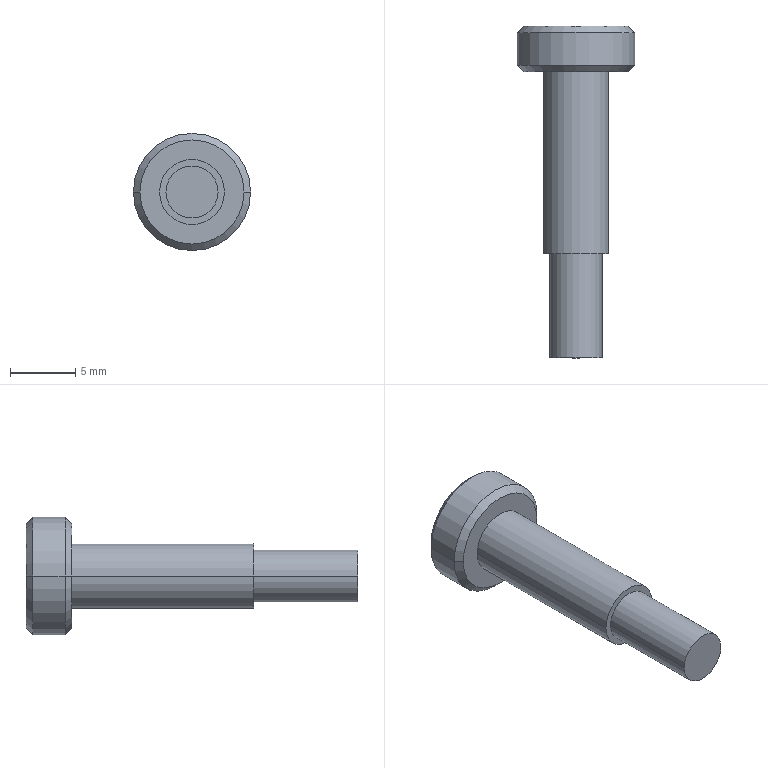Part | SolidWorks | features Attribute 3, Chamfer 1, ICE 1, Revolution 1 | 1 solid | 21 faces | box 9 x 25.5 x 9 mm | volume 575.685 mm3 | plane 11 | cylinder 6 | cone 4 | commonest cylinder face diameters 4 x2 5 x2 9 x2
STEP:
#1=CARTESIAN_POINT('',(4.,22.,0.));
#2=VERTEX_POINT('',#1);
#3=CARTESIAN_POINT('',(-4.,22.,0.));
#4=VERTEX_POINT('',#3);
#5=CARTESIAN_POINT('',(0.,22.,0.));
#6=DIRECTION('',(0.,-1.,0.));
#7=DIRECTION('',(-1.,0.,0.));
#8=AXIS2_PLACEMENT_3D('',#5,#6,#7);
#9=CIRCLE('',#8,4.);
#10=EDGE_CURVE('',#2,#4,#9,.T.);
#11=ORIENTED_EDGE('',*,*,#10,.F.);
#12=CARTESIAN_POINT('',(4.5,22.5,0.));
#13=VERTEX_POINT('',#12);
#14=CARTESIAN_POINT('',(4.,22.,0.));
#15=DIRECTION('',(0.7071,0.7071,0.));
#16=VECTOR('',#15,1000.);
#17=LINE('',#14,#16);
#18=EDGE_CURVE('',#2,#13,#17,.T.);
#19=ORIENTED_EDGE('',*,*,#18,.T.);
#20=CARTESIAN_POINT('',(-4.5,22.5,0.));
#21=VERTEX_POINT('',#20);
#22=CARTESIAN_POINT('',(0.,22.5,0.));
#23=DIRECTION('',(0.,1.,0.));
#24=DIRECTION('',(-1.,0.,0.));
#25=AXIS2_PLACEMENT_3D('',#22,#23,#24);
#26=CIRCLE('',#25,4.5);
#27=EDGE_CURVE('',#21,#13,#26,.T.);
#28=ORIENTED_EDGE('',*,*,#27,.F.);
#29=CARTESIAN_POINT('',(-4.,22.,0.));
#30=DIRECTION('',(-0.7071,0.7071,0.));
#31=VECTOR('',#30,1000.);
#32=LINE('',#29,#31);
#33=EDGE_CURVE('',#4,#21,#32,.T.);
#34=ORIENTED_EDGE('',*,*,#33,.F.);
#35=EDGE_LOOP('',(#11,#19,#28,#34));
#36=FACE_OUTER_BOUND('',#35,.T.);
#37=CARTESIAN_POINT('',(0.,22.,0.));
#38=DIRECTION('',(0.,1.,0.));
#39=DIRECTION('',(-1.,0.,0.));
#40=AXIS2_PLACEMENT_3D('',#37,#38,#39);
#41=CONICAL_SURFACE('',#40,4.,0.7854);
#42=ADVANCED_FACE('',(#36),#41,.T.);
#43=CARTESIAN_POINT('',(-4.,25.5,0.));
#44=VERTEX_POINT('',#43);
#45=CARTESIAN_POINT('',(4.,25.5,0.));
#46=VERTEX_POINT('',#45);
#47=CARTESIAN_POINT('',(0.,25.5,0.));
#48=DIRECTION('',(0.,1.,0.));
#49=DIRECTION('',(1.,0.,0.));
#50=AXIS2_PLACEMENT_3D('',#47,#48,#49);
#51=CIRCLE('',#50,4.);
#52=EDGE_CURVE('',#44,#46,#51,.T.);
#53=ORIENTED_EDGE('',*,*,#52,.F.);
#54=CARTESIAN_POINT('',(-4.5,25.,0.));
#55=VERTEX_POINT('',#54);
#56=CARTESIAN_POINT('',(-4.5,25.,0.));
#57=DIRECTION('',(-0.7071,-0.7071,0.));
#58=VECTOR('',#57,1000.);
#59=LINE('',#56,#58);
#60=EDGE_CURVE('',#44,#55,#59,.T.);
#61=ORIENTED_EDGE('',*,*,#60,.T.);
#62=CARTESIAN_POINT('',(4.5,25.,0.));
#63=VERTEX_POINT('',#62);
#64=CARTESIAN_POINT('',(0.,25.,0.));
#65=DIRECTION('',(0.,-1.,0.));
#66=DIRECTION('',(1.,0.,0.));
#67=AXIS2_PLACEMENT_3D('',#64,#65,#66);
#68=CIRCLE('',#67,4.5);
#69=EDGE_CURVE('',#63,#55,#68,.T.);
#70=ORIENTED_EDGE('',*,*,#69,.F.);
#71=CARTESIAN_POINT('',(4.5,25.,0.));
#72=DIRECTION('',(0.7071,-0.7071,0.));
#73=VECTOR('',#72,1000.);
#74=LINE('',#71,#73);
#75=EDGE_CURVE('',#46,#63,#74,.T.);
#76=ORIENTED_EDGE('',*,*,#75,.F.);
#77=EDGE_LOOP('',(#53,#61,#70,#76));
#78=FACE_OUTER_BOUND('',#77,.T.);
#79=CARTESIAN_POINT('',(0.,25.,0.));
#80=DIRECTION('',(0.,-1.,0.));
#81=DIRECTION('',(1.,0.,0.));
#82=AXIS2_PLACEMENT_3D('',#79,#80,#81);
#83=CONICAL_SURFACE('',#82,4.5,0.7854);
#84=ADVANCED_FACE('',(#78),#83,.T.);
#85=CARTESIAN_POINT('',(2.,8.,0.));
#86=VERTEX_POINT('',#85);
#87=CARTESIAN_POINT('',(-2.,8.,0.));
#88=VERTEX_POINT('',#87);
#89=CARTESIAN_POINT('',(0.,8.,0.));
#90=DIRECTION('',(0.,-1.,0.));
#91=DIRECTION('',(1.,0.,0.));
#92=AXIS2_PLACEMENT_3D('',#89,#90,#91);
#93=CIRCLE('',#92,2.);
#94=EDGE_CURVE('',#86,#88,#93,.T.);
#95=ORIENTED_EDGE('',*,*,#94,.T.);
#96=CARTESIAN_POINT('',(-2.,0.,0.));
#97=VERTEX_POINT('',#96);
#98=CARTESIAN_POINT('',(-2.,0.,0.));
#99=DIRECTION('',(0.,-1.,0.));
#100=VECTOR('',#99,1000.);
#101=LINE('',#98,#100);
#102=EDGE_CURVE('',#88,#97,#101,.T.);
#103=ORIENTED_EDGE('',*,*,#102,.T.);
#104=CARTESIAN_POINT('',(2.,0.,0.));
#105=VERTEX_POINT('',#104);
#106=CARTESIAN_POINT('',(0.,0.,0.));
#107=DIRECTION('',(0.,-1.,0.));
#108=DIRECTION('',(1.,0.,0.));
#109=AXIS2_PLACEMENT_3D('',#106,#107,#108);
#110=CIRCLE('',#109,2.);
#111=EDGE_CURVE('',#105,#97,#110,.T.);
#112=ORIENTED_EDGE('',*,*,#111,.F.);
#113=CARTESIAN_POINT('',(2.,0.,0.));
#114=DIRECTION('',(0.,-1.,0.));
#115=VECTOR('',#114,1000.);
#116=LINE('',#113,#115);
#117=EDGE_CURVE('',#86,#105,#116,.T.);
#118=ORIENTED_EDGE('',*,*,#117,.F.);
#119=EDGE_LOOP('',(#95,#103,#112,#118));
#120=FACE_OUTER_BOUND('',#119,.T.);
#121=CARTESIAN_POINT('',(0.,0.,0.));
#122=DIRECTION('',(0.,-1.,0.));
#123=DIRECTION('',(1.,0.,0.));
#124=AXIS2_PLACEMENT_3D('',#121,#122,#123);
#125=CYLINDRICAL_SURFACE('',#124,2.);
#126=ADVANCED_FACE('',(#120),#125,.T.);
#127=CARTESIAN_POINT('',(2.5,22.,0.));
#128=VERTEX_POINT('',#127);
#129=CARTESIAN_POINT('',(-2.5,22.,0.));
#130=VERTEX_POINT('',#129);
#131=CARTESIAN_POINT('',(0.,22.,0.));
#132=DIRECTION('',(0.,-1.,0.));
#133=DIRECTION('',(1.,0.,0.));
#134=AXIS2_PLACEMENT_3D('',#131,#132,#133);
#135=CIRCLE('',#134,2.5);
#136=EDGE_CURVE('',#128,#130,#135,.T.);
#137=ORIENTED_EDGE('',*,*,#136,.T.);
#138=CARTESIAN_POINT('',(-2.5,8.,0.));
#139=VERTEX_POINT('',#138);
#140=CARTESIAN_POINT('',(-2.5,0.,0.));
#141=DIRECTION('',(0.,-1.,0.));
#142=VECTOR('',#141,1000.);
#143=LINE('',#140,#142);
#144=EDGE_CURVE('',#130,#139,#143,.T.);
#145=ORIENTED_EDGE('',*,*,#144,.T.);
#146=CARTESIAN_POINT('',(2.5,8.,0.));
#147=VERTEX_POINT('',#146);
#148=CARTESIAN_POINT('',(0.,8.,0.));
#149=DIRECTION('',(0.,-1.,0.));
#150=DIRECTION('',(1.,0.,0.));
#151=AXIS2_PLACEMENT_3D('',#148,#149,#150);
#152=CIRCLE('',#151,2.5);
#153=EDGE_CURVE('',#147,#139,#152,.T.);
#154=ORIENTED_EDGE('',*,*,#153,.F.);
#155=CARTESIAN_POINT('',(2.5,0.,0.));
#156=DIRECTION('',(0.,-1.,0.));
#157=VECTOR('',#156,1000.);
#158=LINE('',#155,#157);
#159=EDGE_CURVE('',#128,#147,#158,.T.);
#160=ORIENTED_EDGE('',*,*,#159,.F.);
#161=EDGE_LOOP('',(#137,#145,#154,#160));
#162=FACE_OUTER_BOUND('',#161,.T.);
#163=CARTESIAN_POINT('',(0.,0.,0.));
#164=DIRECTION('',(0.,-1.,0.));
#165=DIRECTION('',(1.,0.,0.));
#166=AXIS2_PLACEMENT_3D('',#163,#164,#165);
#167=CYLINDRICAL_SURFACE('',#166,2.5);
#168=ADVANCED_FACE('',(#162),#167,.T.);
#169=ORIENTED_EDGE('',*,*,#69,.T.);
#170=CARTESIAN_POINT('',(-4.5,0.,0.));
#171=DIRECTION('',(0.,-1.,0.));
#172=VECTOR('',#171,1000.);
#173=LINE('',#170,#172);
#174=EDGE_CURVE('',#55,#21,#173,.T.);
#175=ORIENTED_EDGE('',*,*,#174,.T.);
#176=ORIENTED_EDGE('',*,*,#27,.T.);
#177=CARTESIAN_POINT('',(4.5,0.,0.));
#178=DIRECTION('',(0.,-1.,0.));
#179=VECTOR('',#178,1000.);
#180=LINE('',#177,#179);
#181=EDGE_CURVE('',#63,#13,#180,.T.);
#182=ORIENTED_EDGE('',*,*,#181,.F.);
#183=EDGE_LOOP('',(#169,#175,#176,#182));
#184=FACE_OUTER_BOUND('',#183,.T.);
#185=CARTESIAN_POINT('',(0.,0.,0.));
#186=DIRECTION('',(0.,-1.,0.));
#187=DIRECTION('',(1.,0.,0.));
#188=AXIS2_PLACEMENT_3D('',#185,#186,#187);
#189=CYLINDRICAL_SURFACE('',#188,4.5);
#190=ADVANCED_FACE('',(#184),#189,.T.);
#191=ORIENTED_EDGE('',*,*,#111,.T.);
#192=CARTESIAN_POINT('',(0.,0.,0.));
#193=DIRECTION('',(0.,-1.,0.));
#194=DIRECTION('',(1.,0.,0.));
#195=AXIS2_PLACEMENT_3D('',#192,#193,#194);
#196=CIRCLE('',#195,2.);
#197=EDGE_CURVE('',#97,#105,#196,.T.);
#198=ORIENTED_EDGE('',*,*,#197,.T.);
#199=EDGE_LOOP('',(#191,#198));
#200=FACE_OUTER_BOUND('',#199,.T.);
#201=CARTESIAN_POINT('',(-2.,0.,0.));
#202=DIRECTION('',(0.,1.,0.));
#203=DIRECTION('',(-1.,0.,0.));
#204=AXIS2_PLACEMENT_3D('',#201,#202,#203);
#205=PLANE('',#204);
#206=ADVANCED_FACE('',(#200),#205,.F.);
#207=CARTESIAN_POINT('',(0.,25.5,0.));
#208=DIRECTION('',(0.,1.,0.));
#209=DIRECTION('',(1.,0.,0.));
#210=AXIS2_PLACEMENT_3D('',#207,#208,#209);
#211=CIRCLE('',#210,4.);
#212=EDGE_CURVE('',#46,#44,#211,.T.);
#213=ORIENTED_EDGE('',*,*,#212,.T.);
#214=ORIENTED_EDGE('',*,*,#52,.T.);
#215=EDGE_LOOP('',(#213,#214));
#216=FACE_OUTER_BOUND('',#215,.T.);
#217=CARTESIAN_POINT('',(1.554,25.5,0.7647));
#218=VERTEX_POINT('',#217);
#219=CARTESIAN_POINT('',(1.439,25.5,-0.9635));
#220=VERTEX_POINT('',#219);
#221=CARTESIAN_POINT('',(1.554,25.5,0.7647));
#222=DIRECTION('',(-0.06626,0.,-0.9978));
#223=VECTOR('',#222,1000.);
#224=LINE('',#221,#223);
#225=EDGE_CURVE('',#218,#220,#224,.T.);
#226=ORIENTED_EDGE('',*,*,#225,.F.);
#227=CARTESIAN_POINT('',(0.1148,25.5,1.728));
#228=VERTEX_POINT('',#227);
#229=CARTESIAN_POINT('',(0.1148,25.5,1.728));
#230=DIRECTION('',(0.831,0.,-0.5563));
#231=VECTOR('',#230,1000.);
#232=LINE('',#229,#231);
#233=EDGE_CURVE('',#228,#218,#232,.T.);
#234=ORIENTED_EDGE('',*,*,#233,.F.);
#235=CARTESIAN_POINT('',(-1.439,25.5,0.9635));
#236=VERTEX_POINT('',#235);
#237=CARTESIAN_POINT('',(-1.439,25.5,0.9635));
#238=DIRECTION('',(0.8973,0.,0.4415));
#239=VECTOR('',#238,1000.);
#240=LINE('',#237,#239);
#241=EDGE_CURVE('',#236,#228,#240,.T.);
#242=ORIENTED_EDGE('',*,*,#241,.F.);
#243=CARTESIAN_POINT('',(-1.554,25.5,-0.7647));
#244=VERTEX_POINT('',#243);
#245=CARTESIAN_POINT('',(-1.554,25.5,-0.7647));
#246=DIRECTION('',(0.06626,0.,0.9978));
#247=VECTOR('',#246,1000.);
#248=LINE('',#245,#247);
#249=EDGE_CURVE('',#244,#236,#248,.T.);
#250=ORIENTED_EDGE('',*,*,#249,.F.);
#251=CARTESIAN_POINT('',(-0.1148,25.5,-1.728));
#252=VERTEX_POINT('',#251);
#253=CARTESIAN_POINT('',(-0.1148,25.5,-1.728));
#254=DIRECTION('',(-0.831,0.,0.5563));
#255=VECTOR('',#254,1000.);
#256=LINE('',#253,#255);
#257=EDGE_CURVE('',#252,#244,#256,.T.);
#258=ORIENTED_EDGE('',*,*,#257,.F.);
#259=CARTESIAN_POINT('',(1.439,25.5,-0.9635));
#260=DIRECTION('',(-0.8973,0.,-0.4415));
#261=VECTOR('',#260,1000.);
#262=LINE('',#259,#261);
#263=EDGE_CURVE('',#220,#252,#262,.T.);
#264=ORIENTED_EDGE('',*,*,#263,.F.);
#265=EDGE_LOOP('',(#226,#234,#242,#250,#258,#264));
#266=FACE_BOUND('',#265,.T.);
#267=CARTESIAN_POINT('',(0.,25.5,0.));
#268=DIRECTION('',(0.,-1.,0.));
#269=DIRECTION('',(1.,0.,0.));
#270=AXIS2_PLACEMENT_3D('',#267,#268,#269);
#271=PLANE('',#270);
#272=ADVANCED_FACE('',(#216,#266),#271,.F.);
#273=ORIENTED_EDGE('',*,*,#174,.F.);
#274=CARTESIAN_POINT('',(0.,25.,0.));
#275=DIRECTION('',(0.,-1.,0.));
#276=DIRECTION('',(1.,0.,0.));
#277=AXIS2_PLACEMENT_3D('',#274,#275,#276);
#278=CIRCLE('',#277,4.5);
#279=EDGE_CURVE('',#55,#63,#278,.T.);
#280=ORIENTED_EDGE('',*,*,#279,.T.);
#281=ORIENTED_EDGE('',*,*,#181,.T.);
#282=CARTESIAN_POINT('',(0.,22.5,0.));
#283=DIRECTION('',(0.,1.,0.));
#284=DIRECTION('',(-1.,0.,0.));
#285=AXIS2_PLACEMENT_3D('',#282,#283,#284);
#286=CIRCLE('',#285,4.5);
#287=EDGE_CURVE('',#13,#21,#286,.T.);
#288=ORIENTED_EDGE('',*,*,#287,.T.);
#289=EDGE_LOOP('',(#273,#280,#281,#288));
#290=FACE_OUTER_BOUND('',#289,.T.);
#291=CARTESIAN_POINT('',(0.,0.,0.));
#292=DIRECTION('',(0.,-1.,0.));
#293=DIRECTION('',(1.,0.,0.));
#294=AXIS2_PLACEMENT_3D('',#291,#292,#293);
#295=CYLINDRICAL_SURFACE('',#294,4.5);
#296=ADVANCED_FACE('',(#290),#295,.T.);
#297=CARTESIAN_POINT('',(0.,22.,0.));
#298=DIRECTION('',(0.,-1.,0.));
#299=DIRECTION('',(-1.,0.,0.));
#300=AXIS2_PLACEMENT_3D('',#297,#298,#299);
#301=CIRCLE('',#300,4.);
#302=EDGE_CURVE('',#4,#2,#301,.T.);
#303=ORIENTED_EDGE('',*,*,#302,.T.);
#304=ORIENTED_EDGE('',*,*,#10,.T.);
#305=EDGE_LOOP('',(#303,#304));
#306=FACE_OUTER_BOUND('',#305,.T.);
#307=ORIENTED_EDGE('',*,*,#136,.F.);
#308=CARTESIAN_POINT('',(0.,22.,0.));
#309=DIRECTION('',(0.,-1.,0.));
#310=DIRECTION('',(1.,0.,0.));
#311=AXIS2_PLACEMENT_3D('',#308,#309,#310);
#312=CIRCLE('',#311,2.5);
#313=EDGE_CURVE('',#130,#128,#312,.T.);
#314=ORIENTED_EDGE('',*,*,#313,.F.);
#315=EDGE_LOOP('',(#307,#314));
#316=FACE_BOUND('',#315,.T.);
#317=CARTESIAN_POINT('',(-4.5,22.,0.));
#318=DIRECTION('',(0.,1.,0.));
#319=DIRECTION('',(-1.,0.,0.));
#320=AXIS2_PLACEMENT_3D('',#317,#318,#319);
#321=PLANE('',#320);
#322=ADVANCED_FACE('',(#306,#316),#321,.F.);
#323=ORIENTED_EDGE('',*,*,#144,.F.);
#324=ORIENTED_EDGE('',*,*,#313,.T.);
#325=ORIENTED_EDGE('',*,*,#159,.T.);
#326=CARTESIAN_POINT('',(0.,8.,0.));
#327=DIRECTION('',(0.,-1.,0.));
#328=DIRECTION('',(1.,0.,0.));
#329=AXIS2_PLACEMENT_3D('',#326,#327,#328);
#330=CIRCLE('',#329,2.5);
#331=EDGE_CURVE('',#139,#147,#330,.T.);
#332=ORIENTED_EDGE('',*,*,#331,.F.);
#333=EDGE_LOOP('',(#323,#324,#325,#332));
#334=FACE_OUTER_BOUND('',#333,.T.);
#335=CARTESIAN_POINT('',(0.,0.,0.));
#336=DIRECTION('',(0.,-1.,0.));
#337=DIRECTION('',(1.,0.,0.));
#338=AXIS2_PLACEMENT_3D('',#335,#336,#337);
#339=CYLINDRICAL_SURFACE('',#338,2.5);
#340=ADVANCED_FACE('',(#334),#339,.T.);
#341=ORIENTED_EDGE('',*,*,#94,.F.);
#342=CARTESIAN_POINT('',(0.,8.,0.));
#343=DIRECTION('',(0.,-1.,0.));
#344=DIRECTION('',(1.,0.,0.));
#345=AXIS2_PLACEMENT_3D('',#342,#343,#344);
#346=CIRCLE('',#345,2.);
#347=EDGE_CURVE('',#88,#86,#346,.T.);
#348=ORIENTED_EDGE('',*,*,#347,.F.);
#349=EDGE_LOOP('',(#341,#348));
#350=FACE_BOUND('',#349,.T.);
#351=ORIENTED_EDGE('',*,*,#153,.T.);
#352=ORIENTED_EDGE('',*,*,#331,.T.);
#353=EDGE_LOOP('',(#351,#352));
#354=FACE_OUTER_BOUND('',#353,.T.);
#355=CARTESIAN_POINT('',(-2.5,8.,0.));
#356=DIRECTION('',(0.,1.,0.));
#357=DIRECTION('',(-1.,0.,0.));
#358=AXIS2_PLACEMENT_3D('',#355,#356,#357);
#359=PLANE('',#358);
#360=ADVANCED_FACE('',(#350,#354),#359,.F.);
#361=ORIENTED_EDGE('',*,*,#102,.F.);
#362=ORIENTED_EDGE('',*,*,#347,.T.);
#363=ORIENTED_EDGE('',*,*,#117,.T.);
#364=ORIENTED_EDGE('',*,*,#197,.F.);
#365=EDGE_LOOP('',(#361,#362,#363,#364));
#366=FACE_OUTER_BOUND('',#365,.T.);
#367=CARTESIAN_POINT('',(0.,0.,0.));
#368=DIRECTION('',(0.,-1.,0.));
#369=DIRECTION('',(1.,0.,0.));
#370=AXIS2_PLACEMENT_3D('',#367,#368,#369);
#371=CYLINDRICAL_SURFACE('',#370,2.);
#372=ADVANCED_FACE('',(#366),#371,.T.);
#373=ORIENTED_EDGE('',*,*,#233,.T.);
#374=CARTESIAN_POINT('',(1.554,23.5,0.7647));
#375=VERTEX_POINT('',#374);
#376=CARTESIAN_POINT('',(1.554,23.5,0.7647));
#377=DIRECTION('',(0.,1.,0.));
#378=VECTOR('',#377,1000.);
#379=LINE('',#376,#378);
#380=EDGE_CURVE('',#375,#218,#379,.T.);
#381=ORIENTED_EDGE('',*,*,#380,.F.);
#382=CARTESIAN_POINT('',(0.1148,23.5,1.728));
#383=VERTEX_POINT('',#382);
#384=CARTESIAN_POINT('',(0.1148,23.5,1.728));
#385=DIRECTION('',(0.831,0.,-0.5563));
#386=VECTOR('',#385,1000.);
#387=LINE('',#384,#386);
#388=EDGE_CURVE('',#383,#375,#387,.T.);
#389=ORIENTED_EDGE('',*,*,#388,.F.);
#390=CARTESIAN_POINT('',(0.1148,23.5,1.728));
#391=DIRECTION('',(0.,1.,0.));
#392=VECTOR('',#391,1000.);
#393=LINE('',#390,#392);
#394=EDGE_CURVE('',#383,#228,#393,.T.);
#395=ORIENTED_EDGE('',*,*,#394,.T.);
#396=EDGE_LOOP('',(#373,#381,#389,#395));
#397=FACE_OUTER_BOUND('',#396,.T.);
#398=CARTESIAN_POINT('',(0.1148,23.5,1.728));
#399=DIRECTION('',(0.5563,0.,0.831));
#400=DIRECTION('',(0.831,0.,-0.5563));
#401=AXIS2_PLACEMENT_3D('',#398,#399,#400);
#402=PLANE('',#401);
#403=ADVANCED_FACE('',(#397),#402,.F.);
#404=ORIENTED_EDGE('',*,*,#241,.T.);
#405=ORIENTED_EDGE('',*,*,#394,.F.);
#406=CARTESIAN_POINT('',(-1.439,23.5,0.9635));
#407=VERTEX_POINT('',#406);
#408=CARTESIAN_POINT('',(-1.439,23.5,0.9635));
#409=DIRECTION('',(0.8973,0.,0.4415));
#410=VECTOR('',#409,1000.);
#411=LINE('',#408,#410);
#412=EDGE_CURVE('',#407,#383,#411,.T.);
#413=ORIENTED_EDGE('',*,*,#412,.F.);
#414=CARTESIAN_POINT('',(-1.439,23.5,0.9635));
#415=DIRECTION('',(0.,1.,0.));
#416=VECTOR('',#415,1000.);
#417=LINE('',#414,#416);
#418=EDGE_CURVE('',#407,#236,#417,.T.);
#419=ORIENTED_EDGE('',*,*,#418,.T.);
#420=EDGE_LOOP('',(#404,#405,#413,#419));
#421=FACE_OUTER_BOUND('',#420,.T.);
#422=CARTESIAN_POINT('',(-1.439,23.5,0.9635));
#423=DIRECTION('',(-0.4415,0.,0.8973));
#424=DIRECTION('',(0.8973,0.,0.4415));
#425=AXIS2_PLACEMENT_3D('',#422,#423,#424);
#426=PLANE('',#425);
#427=ADVANCED_FACE('',(#421),#426,.F.);
#428=ORIENTED_EDGE('',*,*,#249,.T.);
#429=ORIENTED_EDGE('',*,*,#418,.F.);
#430=CARTESIAN_POINT('',(-1.554,23.5,-0.7647));
#431=VERTEX_POINT('',#430);
#432=CARTESIAN_POINT('',(-1.554,23.5,-0.7647));
#433=DIRECTION('',(0.06626,0.,0.9978));
#434=VECTOR('',#433,1000.);
#435=LINE('',#432,#434);
#436=EDGE_CURVE('',#431,#407,#435,.T.);
#437=ORIENTED_EDGE('',*,*,#436,.F.);
#438=CARTESIAN_POINT('',(-1.554,23.5,-0.7647));
#439=DIRECTION('',(0.,1.,0.));
#440=VECTOR('',#439,1000.);
#441=LINE('',#438,#440);
#442=EDGE_CURVE('',#431,#244,#441,.T.);
#443=ORIENTED_EDGE('',*,*,#442,.T.);
#444=EDGE_LOOP('',(#428,#429,#437,#443));
#445=FACE_OUTER_BOUND('',#444,.T.);
#446=CARTESIAN_POINT('',(-1.554,23.5,-0.7647));
#447=DIRECTION('',(-0.9978,0.,0.06626));
#448=DIRECTION('',(0.06626,0.,0.9978));
#449=AXIS2_PLACEMENT_3D('',#446,#447,#448);
#450=PLANE('',#449);
#451=ADVANCED_FACE('',(#445),#450,.F.);
#452=ORIENTED_EDGE('',*,*,#257,.T.);
#453=ORIENTED_EDGE('',*,*,#442,.F.);
#454=CARTESIAN_POINT('',(-0.1148,23.5,-1.728));
#455=VERTEX_POINT('',#454);
#456=CARTESIAN_POINT('',(-0.1148,23.5,-1.728));
#457=DIRECTION('',(-0.831,0.,0.5563));
#458=VECTOR('',#457,1000.);
#459=LINE('',#456,#458);
#460=EDGE_CURVE('',#455,#431,#459,.T.);
#461=ORIENTED_EDGE('',*,*,#460,.F.);
#462=CARTESIAN_POINT('',(-0.1148,23.5,-1.728));
#463=DIRECTION('',(0.,1.,0.));
#464=VECTOR('',#463,1000.);
#465=LINE('',#462,#464);
#466=EDGE_CURVE('',#455,#252,#465,.T.);
#467=ORIENTED_EDGE('',*,*,#466,.T.);
#468=EDGE_LOOP('',(#452,#453,#461,#467));
#469=FACE_OUTER_BOUND('',#468,.T.);
#470=CARTESIAN_POINT('',(-0.1148,23.5,-1.728));
#471=DIRECTION('',(-0.5563,0.,-0.831));
#472=DIRECTION('',(-0.831,0.,0.5563));
#473=AXIS2_PLACEMENT_3D('',#470,#471,#472);
#474=PLANE('',#473);
#475=ADVANCED_FACE('',(#469),#474,.F.);
#476=ORIENTED_EDGE('',*,*,#263,.T.);
#477=ORIENTED_EDGE('',*,*,#466,.F.);
#478=CARTESIAN_POINT('',(1.439,23.5,-0.9635));
#479=VERTEX_POINT('',#478);
#480=CARTESIAN_POINT('',(1.439,23.5,-0.9635));
#481=DIRECTION('',(-0.8973,0.,-0.4415));
#482=VECTOR('',#481,1000.);
#483=LINE('',#480,#482);
#484=EDGE_CURVE('',#479,#455,#483,.T.);
#485=ORIENTED_EDGE('',*,*,#484,.F.);
#486=CARTESIAN_POINT('',(1.439,23.5,-0.9635));
#487=DIRECTION('',(0.,1.,0.));
#488=VECTOR('',#487,1000.);
#489=LINE('',#486,#488);
#490=EDGE_CURVE('',#479,#220,#489,.T.);
#491=ORIENTED_EDGE('',*,*,#490,.T.);
#492=EDGE_LOOP('',(#476,#477,#485,#491));
#493=FACE_OUTER_BOUND('',#492,.T.);
#494=CARTESIAN_POINT('',(1.439,23.5,-0.9635));
#495=DIRECTION('',(0.4415,0.,-0.8973));
#496=DIRECTION('',(-0.8973,0.,-0.4415));
#497=AXIS2_PLACEMENT_3D('',#494,#495,#496);
#498=PLANE('',#497);
#499=ADVANCED_FACE('',(#493),#498,.F.);
#500=ORIENTED_EDGE('',*,*,#225,.T.);
#501=ORIENTED_EDGE('',*,*,#490,.F.);
#502=CARTESIAN_POINT('',(1.554,23.5,0.7647));
#503=DIRECTION('',(-0.06626,0.,-0.9978));
#504=VECTOR('',#503,1000.);
#505=LINE('',#502,#504);
#506=EDGE_CURVE('',#375,#479,#505,.T.);
#507=ORIENTED_EDGE('',*,*,#506,.F.);
#508=ORIENTED_EDGE('',*,*,#380,.T.);
#509=EDGE_LOOP('',(#500,#501,#507,#508));
#510=FACE_OUTER_BOUND('',#509,.T.);
#511=CARTESIAN_POINT('',(1.554,23.5,0.7647));
#512=DIRECTION('',(0.9978,0.,-0.06626));
#513=DIRECTION('',(-0.06626,0.,-0.9978));
#514=AXIS2_PLACEMENT_3D('',#511,#512,#513);
#515=PLANE('',#514);
#516=ADVANCED_FACE('',(#510),#515,.F.);
#517=ORIENTED_EDGE('',*,*,#388,.T.);
#518=ORIENTED_EDGE('',*,*,#506,.T.);
#519=ORIENTED_EDGE('',*,*,#484,.T.);
#520=ORIENTED_EDGE('',*,*,#460,.T.);
#521=ORIENTED_EDGE('',*,*,#436,.T.);
#522=ORIENTED_EDGE('',*,*,#412,.T.);
#523=EDGE_LOOP('',(#517,#518,#519,#520,#521,#522));
#524=FACE_OUTER_BOUND('',#523,.T.);
#525=CARTESIAN_POINT('',(0.,23.5,0.));
#526=DIRECTION('',(0.,1.,0.));
#527=DIRECTION('',(0.,0.,1.));
#528=AXIS2_PLACEMENT_3D('',#525,#526,#527);
#529=PLANE('',#528);
#530=ADVANCED_FACE('',(#524),#529,.T.);
#531=ORIENTED_EDGE('',*,*,#60,.F.);
#532=ORIENTED_EDGE('',*,*,#212,.F.);
#533=ORIENTED_EDGE('',*,*,#75,.T.);
#534=ORIENTED_EDGE('',*,*,#279,.F.);
#535=EDGE_LOOP('',(#531,#532,#533,#534));
#536=FACE_OUTER_BOUND('',#535,.T.);
#537=CARTESIAN_POINT('',(0.,25.,0.));
#538=DIRECTION('',(0.,-1.,0.));
#539=DIRECTION('',(1.,0.,0.));
#540=AXIS2_PLACEMENT_3D('',#537,#538,#539);
#541=CONICAL_SURFACE('',#540,4.5,0.7854);
#542=ADVANCED_FACE('',(#536),#541,.T.);
#543=ORIENTED_EDGE('',*,*,#18,.F.);
#544=ORIENTED_EDGE('',*,*,#302,.F.);
#545=ORIENTED_EDGE('',*,*,#33,.T.);
#546=ORIENTED_EDGE('',*,*,#287,.F.);
#547=EDGE_LOOP('',(#543,#544,#545,#546));
#548=FACE_OUTER_BOUND('',#547,.T.);
#549=CARTESIAN_POINT('',(0.,22.,0.));
#550=DIRECTION('',(0.,1.,0.));
#551=DIRECTION('',(-1.,0.,0.));
#552=AXIS2_PLACEMENT_3D('',#549,#550,#551);
#553=CONICAL_SURFACE('',#552,4.,0.7854);
#554=ADVANCED_FACE('',(#548),#553,.T.);
#555=CLOSED_SHELL('',(#42,#84,#126,#168,#190,#206,#272,#296,#322,#340,#360,#372,#403,#427,#451,#475,#499,#516,#530,#542,#554));
#556=MANIFOLD_SOLID_BREP('',#555);
#557=CARTESIAN_POINT('',(0.,0.,0.));
#558=DIRECTION('',(0.,0.,1.));
#559=DIRECTION('',(1.,0.,0.));
#560=AXIS2_PLACEMENT_3D('',#557,#558,#559);
#561=(LENGTH_UNIT()NAMED_UNIT(*)SI_UNIT(.MILLI.,.METRE.));
#562=UNCERTAINTY_MEASURE_WITH_UNIT(LENGTH_MEASURE(0.00001),#561,'','');
#563=(NAMED_UNIT(*)PLANE_ANGLE_UNIT()SI_UNIT($,.RADIAN.));
#564=(NAMED_UNIT(*)SI_UNIT($,.STERADIAN.)SOLID_ANGLE_UNIT());
#565=(GEOMETRIC_REPRESENTATION_CONTEXT(3)GLOBAL_UNCERTAINTY_ASSIGNED_CONTEXT((#562))GLOBAL_UNIT_ASSIGNED_CONTEXT((#561,#563,#564))REPRESENTATION_CONTEXT('',''));
#566=ADVANCED_BREP_SHAPE_REPRESENTATION('',(#556,#560),#565);